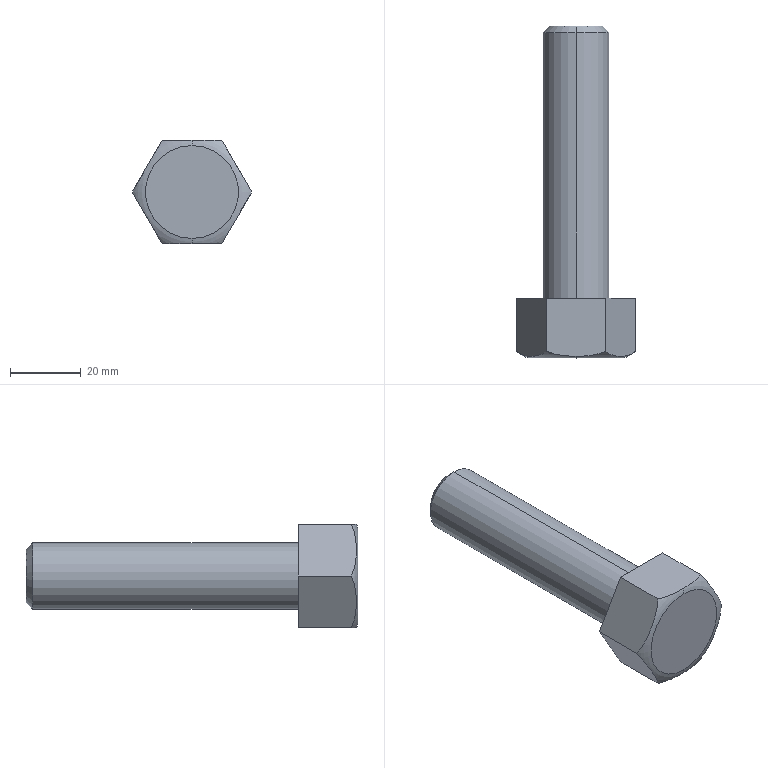Part | SolidWorks | features ICE 1, RevCut 1, Revolution 1, Scale 1 | 1 solid | 15 faces | box 33.75 x 93.75 x 29.228 mm | volume 33536 mm3 | plane 9 | torus 2 | cone 2 | cylinder 2 | commonest cylinder face diameters 18.75 x2
STEP:
#1=CARTESIAN_POINT('',(0.,-17.243,14.614));
#2=VERTEX_POINT('',#1);
#3=CARTESIAN_POINT('',(8.437,-15.803,14.614));
#4=VERTEX_POINT('',#3);
#5=CARTESIAN_POINT('',(0.,-17.243,14.614));
#6=CARTESIAN_POINT('',(0.7213,-17.243,14.614));
#7=CARTESIAN_POINT('',(1.44,-17.222,14.614));
#8=CARTESIAN_POINT('',(2.869,-17.131,14.614));
#9=CARTESIAN_POINT('',(3.581,-17.062,14.614));
#10=CARTESIAN_POINT('',(4.995,-16.856,14.614));
#11=CARTESIAN_POINT('',(5.697,-16.719,14.614));
#12=CARTESIAN_POINT('',(6.739,-16.44,14.614));
#13=CARTESIAN_POINT('',(7.085,-16.334,14.614));
#14=CARTESIAN_POINT('',(7.772,-16.091,14.614));
#15=CARTESIAN_POINT('',(8.109,-15.955,14.614));
#16=CARTESIAN_POINT('',(8.437,-15.803,14.614));
#17=B_SPLINE_CURVE_WITH_KNOTS('',3,(#5,#6,#7,#8,#9,#10,#11,#12,#13,#14,#15,#16),.UNSPECIFIED.,.F.,.F.,(4,2,2,2,2,4),(0.,0.002143,0.004286,0.006428,0.0075,0.008571),.UNSPECIFIED.);
#18=EDGE_CURVE('',#2,#4,#17,.T.);
#19=ORIENTED_EDGE('',*,*,#18,.F.);
#20=CARTESIAN_POINT('',(0.,-17.678,13.125));
#21=VERTEX_POINT('',#20);
#22=CARTESIAN_POINT('',(0.,-10.3,11.78));
#23=DIRECTION('',(1.,0.,0.));
#24=DIRECTION('',(0.,0.,-1.));
#25=AXIS2_PLACEMENT_3D('',#22,#23,#24);
#26=CIRCLE('',#25,7.5);
#27=EDGE_CURVE('',#2,#21,#26,.T.);
#28=ORIENTED_EDGE('',*,*,#27,.T.);
#29=CARTESIAN_POINT('',(0.,-17.678,-13.125));
#30=VERTEX_POINT('',#29);
#31=CARTESIAN_POINT('',(0.,-17.678,0.));
#32=DIRECTION('',(0.,-1.,0.));
#33=DIRECTION('',(0.,0.,-1.));
#34=AXIS2_PLACEMENT_3D('',#31,#32,#33);
#35=CIRCLE('',#34,13.125);
#36=EDGE_CURVE('',#30,#21,#35,.T.);
#37=ORIENTED_EDGE('',*,*,#36,.F.);
#38=CARTESIAN_POINT('',(0.,-17.243,-14.614));
#39=VERTEX_POINT('',#38);
#40=CARTESIAN_POINT('',(0.,-10.3,-11.78));
#41=DIRECTION('',(-1.,0.,0.));
#42=DIRECTION('',(0.,0.,1.));
#43=AXIS2_PLACEMENT_3D('',#40,#41,#42);
#44=CIRCLE('',#43,7.5);
#45=EDGE_CURVE('',#39,#30,#44,.T.);
#46=ORIENTED_EDGE('',*,*,#45,.F.);
#47=CARTESIAN_POINT('',(8.438,-15.803,-14.614));
#48=VERTEX_POINT('',#47);
#49=CARTESIAN_POINT('',(8.438,-15.803,-14.614));
#50=CARTESIAN_POINT('',(7.784,-16.105,-14.614));
#51=CARTESIAN_POINT('',(7.108,-16.339,-14.614));
#52=CARTESIAN_POINT('',(5.723,-16.713,-14.614));
#53=CARTESIAN_POINT('',(5.012,-16.853,-14.614));
#54=CARTESIAN_POINT('',(3.588,-17.061,-14.614));
#55=CARTESIAN_POINT('',(2.874,-17.131,-14.614));
#56=CARTESIAN_POINT('',(1.798,-17.199,-14.614));
#57=CARTESIAN_POINT('',(1.439,-17.216,-14.614));
#58=CARTESIAN_POINT('',(0.9,-17.232,-14.614));
#59=CARTESIAN_POINT('',(0.7202,-17.237,-14.614));
#60=CARTESIAN_POINT('',(0.3603,-17.242,-14.614));
#61=CARTESIAN_POINT('',(0.179,-17.243,-14.614));
#62=CARTESIAN_POINT('',(0.,-17.243,-14.614));
#63=B_SPLINE_CURVE_WITH_KNOTS('',3,(#49,#50,#51,#52,#53,#54,#55,#56,#57,#58,#59,#60,#61,#62),.UNSPECIFIED.,.F.,.F.,(4,2,2,2,2,2,4),(0.05427,0.05639,0.05852,0.06065,0.06171,0.06224,0.06278),.UNSPECIFIED.);
#64=EDGE_CURVE('',#48,#39,#63,.T.);
#65=ORIENTED_EDGE('',*,*,#64,.F.);
#66=CARTESIAN_POINT('',(16.875,-15.803,0.));
#67=VERTEX_POINT('',#66);
#68=CARTESIAN_POINT('',(16.875,-15.803,0.));
#69=CARTESIAN_POINT('',(16.545,-16.109,-0.5716));
#70=CARTESIAN_POINT('',(16.206,-16.342,-1.159));
#71=CARTESIAN_POINT('',(15.514,-16.715,-2.357));
#72=CARTESIAN_POINT('',(15.162,-16.853,-2.967));
#73=CARTESIAN_POINT('',(14.449,-17.061,-4.201));
#74=CARTESIAN_POINT('',(14.09,-17.132,-4.824));
#75=CARTESIAN_POINT('',(13.373,-17.222,-6.065));
#76=CARTESIAN_POINT('',(13.016,-17.243,-6.685));
#77=CARTESIAN_POINT('',(12.3,-17.243,-7.923));
#78=CARTESIAN_POINT('',(11.943,-17.223,-8.542));
#79=CARTESIAN_POINT('',(11.229,-17.133,-9.78));
#80=CARTESIAN_POINT('',(10.872,-17.063,-10.398));
#81=CARTESIAN_POINT('',(10.159,-16.856,-11.633));
#82=CARTESIAN_POINT('',(9.802,-16.717,-12.25));
#83=CARTESIAN_POINT('',(9.107,-16.343,-13.454));
#84=CARTESIAN_POINT('',(8.767,-16.108,-14.043));
#85=CARTESIAN_POINT('',(8.438,-15.803,-14.614));
#86=B_SPLINE_CURVE_WITH_KNOTS('',3,(#68,#69,#70,#71,#72,#73,#74,#75,#76,#77,#78,#79,#80,#81,#82,#83,#84,#85),.UNSPECIFIED.,.F.,.F.,(4,2,2,2,2,2,2,2,4),(0.00000047,0.002148,0.004296,0.006444,0.008592,0.01074,0.01289,0.01504,0.01718),.UNSPECIFIED.);
#87=EDGE_CURVE('',#67,#48,#86,.T.);
#88=ORIENTED_EDGE('',*,*,#87,.F.);
#89=CARTESIAN_POINT('',(8.437,-15.803,14.614));
#90=CARTESIAN_POINT('',(8.768,-16.109,14.043));
#91=CARTESIAN_POINT('',(9.107,-16.342,13.455));
#92=CARTESIAN_POINT('',(9.798,-16.715,12.257));
#93=CARTESIAN_POINT('',(10.15,-16.853,11.648));
#94=CARTESIAN_POINT('',(10.863,-17.061,10.413));
#95=CARTESIAN_POINT('',(11.223,-17.132,9.79));
#96=CARTESIAN_POINT('',(11.939,-17.222,8.549));
#97=CARTESIAN_POINT('',(12.297,-17.243,7.93));
#98=CARTESIAN_POINT('',(13.012,-17.243,6.691));
#99=CARTESIAN_POINT('',(13.369,-17.223,6.072));
#100=CARTESIAN_POINT('',(14.084,-17.133,4.835));
#101=CARTESIAN_POINT('',(14.441,-17.063,4.217));
#102=CARTESIAN_POINT('',(15.154,-16.856,2.982));
#103=CARTESIAN_POINT('',(15.51,-16.717,2.364));
#104=CARTESIAN_POINT('',(16.205,-16.343,1.16));
#105=CARTESIAN_POINT('',(16.545,-16.108,0.5709));
#106=CARTESIAN_POINT('',(16.875,-15.803,0.));
#107=B_SPLINE_CURVE_WITH_KNOTS('',3,(#89,#90,#91,#92,#93,#94,#95,#96,#97,#98,#99,#100,#101,#102,#103,#104,#105,#106),.UNSPECIFIED.,.F.,.F.,(4,2,2,2,2,2,2,2,4),(0.00000047,0.002148,0.004296,0.006444,0.008592,0.01074,0.01289,0.01504,0.01718),.UNSPECIFIED.);
#108=EDGE_CURVE('',#4,#67,#107,.T.);
#109=ORIENTED_EDGE('',*,*,#108,.F.);
#110=EDGE_LOOP('',(#19,#28,#37,#46,#65,#88,#109));
#111=FACE_OUTER_BOUND('',#110,.T.);
#112=CARTESIAN_POINT('',(0.,-10.3,0.));
#113=DIRECTION('',(0.,-1.,0.));
#114=DIRECTION('',(0.,0.,-1.));
#115=AXIS2_PLACEMENT_3D('',#112,#113,#114);
#116=TOROIDAL_SURFACE('',#115,11.78,7.5);
#117=ADVANCED_FACE('',(#111),#116,.T.);
#118=CARTESIAN_POINT('',(0.,76.072,7.5));
#119=VERTEX_POINT('',#118);
#120=CARTESIAN_POINT('',(0.,76.072,-7.5));
#121=VERTEX_POINT('',#120);
#122=CARTESIAN_POINT('',(0.,76.072,0.));
#123=DIRECTION('',(0.,1.,0.));
#124=DIRECTION('',(0.,0.,1.));
#125=AXIS2_PLACEMENT_3D('',#122,#123,#124);
#126=CIRCLE('',#125,7.5);
#127=EDGE_CURVE('',#119,#121,#126,.T.);
#128=ORIENTED_EDGE('',*,*,#127,.F.);
#129=CARTESIAN_POINT('',(0.,74.197,9.375));
#130=VERTEX_POINT('',#129);
#131=CARTESIAN_POINT('',(0.,74.197,9.375));
#132=DIRECTION('',(0.,-0.7071,0.7071));
#133=VECTOR('',#132,1000.);
#134=LINE('',#131,#133);
#135=EDGE_CURVE('',#119,#130,#134,.T.);
#136=ORIENTED_EDGE('',*,*,#135,.T.);
#137=CARTESIAN_POINT('',(0.,74.197,-9.375));
#138=VERTEX_POINT('',#137);
#139=CARTESIAN_POINT('',(0.,74.197,0.));
#140=DIRECTION('',(0.,1.,0.));
#141=DIRECTION('',(0.,0.,1.));
#142=AXIS2_PLACEMENT_3D('',#139,#140,#141);
#143=CIRCLE('',#142,9.375);
#144=EDGE_CURVE('',#130,#138,#143,.T.);
#145=ORIENTED_EDGE('',*,*,#144,.T.);
#146=CARTESIAN_POINT('',(0.,74.197,-9.375));
#147=DIRECTION('',(0.,-0.7071,-0.7071));
#148=VECTOR('',#147,1000.);
#149=LINE('',#146,#148);
#150=EDGE_CURVE('',#121,#138,#149,.T.);
#151=ORIENTED_EDGE('',*,*,#150,.F.);
#152=EDGE_LOOP('',(#128,#136,#145,#151));
#153=FACE_OUTER_BOUND('',#152,.T.);
#154=CARTESIAN_POINT('',(0.,74.197,0.));
#155=DIRECTION('',(0.,-1.,0.));
#156=DIRECTION('',(0.,0.,-1.));
#157=AXIS2_PLACEMENT_3D('',#154,#155,#156);
#158=CONICAL_SURFACE('',#157,9.375,0.7854);
#159=ADVANCED_FACE('',(#153),#158,.T.);
#160=CARTESIAN_POINT('',(0.,-0.803,9.375));
#161=VERTEX_POINT('',#160);
#162=CARTESIAN_POINT('',(0.,-0.803,-9.375));
#163=VERTEX_POINT('',#162);
#164=CARTESIAN_POINT('',(0.,-0.803,0.));
#165=DIRECTION('',(0.,1.,0.));
#166=DIRECTION('',(0.,0.,1.));
#167=AXIS2_PLACEMENT_3D('',#164,#165,#166);
#168=CIRCLE('',#167,9.375);
#169=EDGE_CURVE('',#161,#163,#168,.T.);
#170=ORIENTED_EDGE('',*,*,#169,.T.);
#171=CARTESIAN_POINT('',(0.,76.072,-9.375));
#172=DIRECTION('',(0.,1.,0.));
#173=VECTOR('',#172,1000.);
#174=LINE('',#171,#173);
#175=EDGE_CURVE('',#163,#138,#174,.T.);
#176=ORIENTED_EDGE('',*,*,#175,.T.);
#177=ORIENTED_EDGE('',*,*,#144,.F.);
#178=CARTESIAN_POINT('',(0.,76.072,9.375));
#179=DIRECTION('',(0.,1.,0.));
#180=VECTOR('',#179,1000.);
#181=LINE('',#178,#180);
#182=EDGE_CURVE('',#161,#130,#181,.T.);
#183=ORIENTED_EDGE('',*,*,#182,.F.);
#184=EDGE_LOOP('',(#170,#176,#177,#183));
#185=FACE_OUTER_BOUND('',#184,.T.);
#186=CARTESIAN_POINT('',(0.,76.072,0.));
#187=DIRECTION('',(0.,1.,0.));
#188=DIRECTION('',(0.,0.,1.));
#189=AXIS2_PLACEMENT_3D('',#186,#187,#188);
#190=CYLINDRICAL_SURFACE('',#189,9.375);
#191=ADVANCED_FACE('',(#185),#190,.T.);
#192=CARTESIAN_POINT('',(16.875,-0.803,0.));
#193=VERTEX_POINT('',#192);
#194=CARTESIAN_POINT('',(16.875,1.072,0.));
#195=DIRECTION('',(0.,-1.,0.));
#196=VECTOR('',#195,1000.);
#197=LINE('',#194,#196);
#198=EDGE_CURVE('',#193,#67,#197,.T.);
#199=ORIENTED_EDGE('',*,*,#198,.T.);
#200=ORIENTED_EDGE('',*,*,#87,.T.);
#201=CARTESIAN_POINT('',(8.438,-0.803,-14.614));
#202=VERTEX_POINT('',#201);
#203=CARTESIAN_POINT('',(8.438,1.072,-14.614));
#204=DIRECTION('',(0.,-1.,0.));
#205=VECTOR('',#204,1000.);
#206=LINE('',#203,#205);
#207=EDGE_CURVE('',#202,#48,#206,.T.);
#208=ORIENTED_EDGE('',*,*,#207,.F.);
#209=CARTESIAN_POINT('',(16.875,-0.803,0.));
#210=DIRECTION('',(0.5,0.,0.866));
#211=VECTOR('',#210,1000.);
#212=LINE('',#209,#211);
#213=EDGE_CURVE('',#202,#193,#212,.T.);
#214=ORIENTED_EDGE('',*,*,#213,.T.);
#215=EDGE_LOOP('',(#199,#200,#208,#214));
#216=FACE_OUTER_BOUND('',#215,.T.);
#217=CARTESIAN_POINT('',(8.438,1.072,-14.614));
#218=DIRECTION('',(0.866,0.,-0.5));
#219=DIRECTION('',(-0.5,0.,-0.866));
#220=AXIS2_PLACEMENT_3D('',#217,#218,#219);
#221=PLANE('',#220);
#222=ADVANCED_FACE('',(#216),#221,.T.);
#223=ORIENTED_EDGE('',*,*,#207,.T.);
#224=ORIENTED_EDGE('',*,*,#64,.T.);
#225=CARTESIAN_POINT('',(-8.437,-15.803,-14.614));
#226=VERTEX_POINT('',#225);
#227=CARTESIAN_POINT('',(0.,-17.243,-14.614));
#228=CARTESIAN_POINT('',(-0.7213,-17.243,-14.614));
#229=CARTESIAN_POINT('',(-1.44,-17.222,-14.614));
#230=CARTESIAN_POINT('',(-2.869,-17.131,-14.614));
#231=CARTESIAN_POINT('',(-3.581,-17.062,-14.614));
#232=CARTESIAN_POINT('',(-4.995,-16.856,-14.614));
#233=CARTESIAN_POINT('',(-5.697,-16.719,-14.614));
#234=CARTESIAN_POINT('',(-6.739,-16.44,-14.614));
#235=CARTESIAN_POINT('',(-7.085,-16.334,-14.614));
#236=CARTESIAN_POINT('',(-7.772,-16.091,-14.614));
#237=CARTESIAN_POINT('',(-8.109,-15.955,-14.614));
#238=CARTESIAN_POINT('',(-8.437,-15.803,-14.614));
#239=B_SPLINE_CURVE_WITH_KNOTS('',3,(#227,#228,#229,#230,#231,#232,#233,#234,#235,#236,#237,#238),.UNSPECIFIED.,.F.,.F.,(4,2,2,2,2,4),(0.,0.002143,0.004286,0.006428,0.0075,0.008571),.UNSPECIFIED.);
#240=EDGE_CURVE('',#39,#226,#239,.T.);
#241=ORIENTED_EDGE('',*,*,#240,.T.);
#242=CARTESIAN_POINT('',(-8.437,-0.803,-14.614));
#243=VERTEX_POINT('',#242);
#244=CARTESIAN_POINT('',(-8.437,1.072,-14.614));
#245=DIRECTION('',(0.,-1.,0.));
#246=VECTOR('',#245,1000.);
#247=LINE('',#244,#246);
#248=EDGE_CURVE('',#243,#226,#247,.T.);
#249=ORIENTED_EDGE('',*,*,#248,.F.);
#250=CARTESIAN_POINT('',(16.875,-0.803,-14.614));
#251=DIRECTION('',(1.,0.,0.));
#252=VECTOR('',#251,1000.);
#253=LINE('',#250,#252);
#254=EDGE_CURVE('',#243,#202,#253,.T.);
#255=ORIENTED_EDGE('',*,*,#254,.T.);
#256=EDGE_LOOP('',(#223,#224,#241,#249,#255));
#257=FACE_OUTER_BOUND('',#256,.T.);
#258=CARTESIAN_POINT('',(-8.437,1.072,-14.614));
#259=DIRECTION('',(0.,0.,-1.));
#260=DIRECTION('',(-1.,0.,0.));
#261=AXIS2_PLACEMENT_3D('',#258,#259,#260);
#262=PLANE('',#261);
#263=ADVANCED_FACE('',(#257),#262,.T.);
#264=ORIENTED_EDGE('',*,*,#248,.T.);
#265=CARTESIAN_POINT('',(-16.875,-15.803,0.));
#266=VERTEX_POINT('',#265);
#267=CARTESIAN_POINT('',(-8.437,-15.803,-14.614));
#268=CARTESIAN_POINT('',(-8.768,-16.109,-14.043));
#269=CARTESIAN_POINT('',(-9.107,-16.342,-13.455));
#270=CARTESIAN_POINT('',(-9.798,-16.715,-12.257));
#271=CARTESIAN_POINT('',(-10.15,-16.853,-11.648));
#272=CARTESIAN_POINT('',(-10.863,-17.061,-10.413));
#273=CARTESIAN_POINT('',(-11.223,-17.132,-9.79));
#274=CARTESIAN_POINT('',(-11.939,-17.222,-8.549));
#275=CARTESIAN_POINT('',(-12.297,-17.243,-7.93));
#276=CARTESIAN_POINT('',(-13.012,-17.243,-6.691));
#277=CARTESIAN_POINT('',(-13.369,-17.223,-6.072));
#278=CARTESIAN_POINT('',(-14.084,-17.133,-4.835));
#279=CARTESIAN_POINT('',(-14.441,-17.063,-4.217));
#280=CARTESIAN_POINT('',(-15.154,-16.856,-2.982));
#281=CARTESIAN_POINT('',(-15.51,-16.717,-2.364));
#282=CARTESIAN_POINT('',(-16.205,-16.343,-1.16));
#283=CARTESIAN_POINT('',(-16.545,-16.108,-0.5709));
#284=CARTESIAN_POINT('',(-16.875,-15.803,0.));
#285=B_SPLINE_CURVE_WITH_KNOTS('',3,(#267,#268,#269,#270,#271,#272,#273,#274,#275,#276,#277,#278,#279,#280,#281,#282,#283,#284),.UNSPECIFIED.,.F.,.F.,(4,2,2,2,2,2,2,2,4),(0.00000047,0.002148,0.004296,0.006444,0.008592,0.01074,0.01289,0.01504,0.01718),.UNSPECIFIED.);
#286=EDGE_CURVE('',#226,#266,#285,.T.);
#287=ORIENTED_EDGE('',*,*,#286,.T.);
#288=CARTESIAN_POINT('',(-16.875,-0.803,0.));
#289=VERTEX_POINT('',#288);
#290=CARTESIAN_POINT('',(-16.875,1.072,0.));
#291=DIRECTION('',(0.,-1.,0.));
#292=VECTOR('',#291,1000.);
#293=LINE('',#290,#292);
#294=EDGE_CURVE('',#289,#266,#293,.T.);
#295=ORIENTED_EDGE('',*,*,#294,.F.);
#296=CARTESIAN_POINT('',(-8.437,-0.803,-14.614));
#297=DIRECTION('',(0.5,0.,-0.866));
#298=VECTOR('',#297,1000.);
#299=LINE('',#296,#298);
#300=EDGE_CURVE('',#289,#243,#299,.T.);
#301=ORIENTED_EDGE('',*,*,#300,.T.);
#302=EDGE_LOOP('',(#264,#287,#295,#301));
#303=FACE_OUTER_BOUND('',#302,.T.);
#304=CARTESIAN_POINT('',(-16.875,1.072,0.));
#305=DIRECTION('',(-0.866,0.,-0.5));
#306=DIRECTION('',(-0.5,0.,0.866));
#307=AXIS2_PLACEMENT_3D('',#304,#305,#306);
#308=PLANE('',#307);
#309=ADVANCED_FACE('',(#303),#308,.T.);
#310=ORIENTED_EDGE('',*,*,#294,.T.);
#311=CARTESIAN_POINT('',(-8.438,-15.803,14.614));
#312=VERTEX_POINT('',#311);
#313=CARTESIAN_POINT('',(-16.875,-15.803,0.));
#314=CARTESIAN_POINT('',(-16.545,-16.109,0.5716));
#315=CARTESIAN_POINT('',(-16.206,-16.342,1.159));
#316=CARTESIAN_POINT('',(-15.514,-16.715,2.357));
#317=CARTESIAN_POINT('',(-15.162,-16.853,2.967));
#318=CARTESIAN_POINT('',(-14.449,-17.061,4.201));
#319=CARTESIAN_POINT('',(-14.09,-17.132,4.824));
#320=CARTESIAN_POINT('',(-13.373,-17.222,6.065));
#321=CARTESIAN_POINT('',(-13.016,-17.243,6.685));
#322=CARTESIAN_POINT('',(-12.3,-17.243,7.923));
#323=CARTESIAN_POINT('',(-11.943,-17.223,8.542));
#324=CARTESIAN_POINT('',(-11.229,-17.133,9.78));
#325=CARTESIAN_POINT('',(-10.872,-17.063,10.398));
#326=CARTESIAN_POINT('',(-10.159,-16.856,11.633));
#327=CARTESIAN_POINT('',(-9.802,-16.717,12.25));
#328=CARTESIAN_POINT('',(-9.107,-16.343,13.454));
#329=CARTESIAN_POINT('',(-8.767,-16.108,14.043));
#330=CARTESIAN_POINT('',(-8.438,-15.803,14.614));
#331=B_SPLINE_CURVE_WITH_KNOTS('',3,(#313,#314,#315,#316,#317,#318,#319,#320,#321,#322,#323,#324,#325,#326,#327,#328,#329,#330),.UNSPECIFIED.,.F.,.F.,(4,2,2,2,2,2,2,2,4),(0.00000047,0.002148,0.004296,0.006444,0.008592,0.01074,0.01289,0.01504,0.01718),.UNSPECIFIED.);
#332=EDGE_CURVE('',#266,#312,#331,.T.);
#333=ORIENTED_EDGE('',*,*,#332,.T.);
#334=CARTESIAN_POINT('',(-8.438,-0.803,14.614));
#335=VERTEX_POINT('',#334);
#336=CARTESIAN_POINT('',(-8.438,1.072,14.614));
#337=DIRECTION('',(0.,-1.,0.));
#338=VECTOR('',#337,1000.);
#339=LINE('',#336,#338);
#340=EDGE_CURVE('',#335,#312,#339,.T.);
#341=ORIENTED_EDGE('',*,*,#340,.F.);
#342=CARTESIAN_POINT('',(-8.438,-0.803,14.614));
#343=DIRECTION('',(-0.5,0.,-0.866));
#344=VECTOR('',#343,1000.);
#345=LINE('',#342,#344);
#346=EDGE_CURVE('',#335,#289,#345,.T.);
#347=ORIENTED_EDGE('',*,*,#346,.T.);
#348=EDGE_LOOP('',(#310,#333,#341,#347));
#349=FACE_OUTER_BOUND('',#348,.T.);
#350=CARTESIAN_POINT('',(-8.438,1.072,14.614));
#351=DIRECTION('',(-0.866,0.,0.5));
#352=DIRECTION('',(0.5,0.,0.866));
#353=AXIS2_PLACEMENT_3D('',#350,#351,#352);
#354=PLANE('',#353);
#355=ADVANCED_FACE('',(#349),#354,.T.);
#356=ORIENTED_EDGE('',*,*,#340,.T.);
#357=CARTESIAN_POINT('',(-8.438,-15.803,14.614));
#358=CARTESIAN_POINT('',(-7.784,-16.105,14.614));
#359=CARTESIAN_POINT('',(-7.108,-16.339,14.614));
#360=CARTESIAN_POINT('',(-5.723,-16.713,14.614));
#361=CARTESIAN_POINT('',(-5.012,-16.853,14.614));
#362=CARTESIAN_POINT('',(-3.588,-17.061,14.614));
#363=CARTESIAN_POINT('',(-2.874,-17.131,14.614));
#364=CARTESIAN_POINT('',(-1.798,-17.199,14.614));
#365=CARTESIAN_POINT('',(-1.439,-17.216,14.614));
#366=CARTESIAN_POINT('',(-0.9,-17.232,14.614));
#367=CARTESIAN_POINT('',(-0.7202,-17.237,14.614));
#368=CARTESIAN_POINT('',(-0.3603,-17.242,14.614));
#369=CARTESIAN_POINT('',(-0.179,-17.243,14.614));
#370=CARTESIAN_POINT('',(0.,-17.243,14.614));
#371=B_SPLINE_CURVE_WITH_KNOTS('',3,(#357,#358,#359,#360,#361,#362,#363,#364,#365,#366,#367,#368,#369,#370),.UNSPECIFIED.,.F.,.F.,(4,2,2,2,2,2,4),(0.05427,0.05639,0.05852,0.06065,0.06171,0.06224,0.06278),.UNSPECIFIED.);
#372=EDGE_CURVE('',#312,#2,#371,.T.);
#373=ORIENTED_EDGE('',*,*,#372,.T.);
#374=ORIENTED_EDGE('',*,*,#18,.T.);
#375=CARTESIAN_POINT('',(8.437,-0.803,14.614));
#376=VERTEX_POINT('',#375);
#377=CARTESIAN_POINT('',(8.437,1.072,14.614));
#378=DIRECTION('',(0.,-1.,0.));
#379=VECTOR('',#378,1000.);
#380=LINE('',#377,#379);
#381=EDGE_CURVE('',#376,#4,#380,.T.);
#382=ORIENTED_EDGE('',*,*,#381,.F.);
#383=CARTESIAN_POINT('',(16.875,-0.803,14.614));
#384=DIRECTION('',(-1.,0.,0.));
#385=VECTOR('',#384,1000.);
#386=LINE('',#383,#385);
#387=EDGE_CURVE('',#376,#335,#386,.T.);
#388=ORIENTED_EDGE('',*,*,#387,.T.);
#389=EDGE_LOOP('',(#356,#373,#374,#382,#388));
#390=FACE_OUTER_BOUND('',#389,.T.);
#391=CARTESIAN_POINT('',(8.437,1.072,14.614));
#392=DIRECTION('',(0.,0.,1.));
#393=DIRECTION('',(1.,0.,0.));
#394=AXIS2_PLACEMENT_3D('',#391,#392,#393);
#395=PLANE('',#394);
#396=ADVANCED_FACE('',(#390),#395,.T.);
#397=ORIENTED_EDGE('',*,*,#381,.T.);
#398=ORIENTED_EDGE('',*,*,#108,.T.);
#399=ORIENTED_EDGE('',*,*,#198,.F.);
#400=CARTESIAN_POINT('',(16.875,-0.803,0.));
#401=DIRECTION('',(-0.5,0.,0.866));
#402=VECTOR('',#401,1000.);
#403=LINE('',#400,#402);
#404=EDGE_CURVE('',#193,#376,#403,.T.);
#405=ORIENTED_EDGE('',*,*,#404,.T.);
#406=EDGE_LOOP('',(#397,#398,#399,#405));
#407=FACE_OUTER_BOUND('',#406,.T.);
#408=CARTESIAN_POINT('',(16.875,1.072,0.));
#409=DIRECTION('',(0.866,0.,0.5));
#410=DIRECTION('',(0.5,0.,-0.866));
#411=AXIS2_PLACEMENT_3D('',#408,#409,#410);
#412=PLANE('',#411);
#413=ADVANCED_FACE('',(#407),#412,.T.);
#414=ORIENTED_EDGE('',*,*,#169,.F.);
#415=CARTESIAN_POINT('',(0.,-0.803,0.));
#416=DIRECTION('',(0.,1.,0.));
#417=DIRECTION('',(0.,0.,1.));
#418=AXIS2_PLACEMENT_3D('',#415,#416,#417);
#419=CIRCLE('',#418,9.375);
#420=EDGE_CURVE('',#163,#161,#419,.T.);
#421=ORIENTED_EDGE('',*,*,#420,.F.);
#422=EDGE_LOOP('',(#414,#421));
#423=FACE_BOUND('',#422,.T.);
#424=ORIENTED_EDGE('',*,*,#213,.F.);
#425=ORIENTED_EDGE('',*,*,#254,.F.);
#426=ORIENTED_EDGE('',*,*,#300,.F.);
#427=ORIENTED_EDGE('',*,*,#346,.F.);
#428=ORIENTED_EDGE('',*,*,#387,.F.);
#429=ORIENTED_EDGE('',*,*,#404,.F.);
#430=EDGE_LOOP('',(#424,#425,#426,#427,#428,#429));
#431=FACE_OUTER_BOUND('',#430,.T.);
#432=CARTESIAN_POINT('',(16.875,-0.803,0.));
#433=DIRECTION('',(0.,-1.,0.));
#434=DIRECTION('',(0.,0.,-1.));
#435=AXIS2_PLACEMENT_3D('',#432,#433,#434);
#436=PLANE('',#435);
#437=ADVANCED_FACE('',(#423,#431),#436,.F.);
#438=ORIENTED_EDGE('',*,*,#175,.F.);
#439=ORIENTED_EDGE('',*,*,#420,.T.);
#440=ORIENTED_EDGE('',*,*,#182,.T.);
#441=CARTESIAN_POINT('',(0.,74.197,0.));
#442=DIRECTION('',(0.,1.,0.));
#443=DIRECTION('',(0.,0.,1.));
#444=AXIS2_PLACEMENT_3D('',#441,#442,#443);
#445=CIRCLE('',#444,9.375);
#446=EDGE_CURVE('',#138,#130,#445,.T.);
#447=ORIENTED_EDGE('',*,*,#446,.F.);
#448=EDGE_LOOP('',(#438,#439,#440,#447));
#449=FACE_OUTER_BOUND('',#448,.T.);
#450=CARTESIAN_POINT('',(0.,76.072,0.));
#451=DIRECTION('',(0.,1.,0.));
#452=DIRECTION('',(0.,0.,1.));
#453=AXIS2_PLACEMENT_3D('',#450,#451,#452);
#454=CYLINDRICAL_SURFACE('',#453,9.375);
#455=ADVANCED_FACE('',(#449),#454,.T.);
#456=ORIENTED_EDGE('',*,*,#135,.F.);
#457=CARTESIAN_POINT('',(0.,76.072,0.));
#458=DIRECTION('',(0.,1.,0.));
#459=DIRECTION('',(0.,0.,1.));
#460=AXIS2_PLACEMENT_3D('',#457,#458,#459);
#461=CIRCLE('',#460,7.5);
#462=EDGE_CURVE('',#121,#119,#461,.T.);
#463=ORIENTED_EDGE('',*,*,#462,.F.);
#464=ORIENTED_EDGE('',*,*,#150,.T.);
#465=ORIENTED_EDGE('',*,*,#446,.T.);
#466=EDGE_LOOP('',(#456,#463,#464,#465));
#467=FACE_OUTER_BOUND('',#466,.T.);
#468=CARTESIAN_POINT('',(0.,74.197,0.));
#469=DIRECTION('',(0.,-1.,0.));
#470=DIRECTION('',(0.,0.,-1.));
#471=AXIS2_PLACEMENT_3D('',#468,#469,#470);
#472=CONICAL_SURFACE('',#471,9.375,0.7854);
#473=ADVANCED_FACE('',(#467),#472,.T.);
#474=ORIENTED_EDGE('',*,*,#462,.T.);
#475=ORIENTED_EDGE('',*,*,#127,.T.);
#476=EDGE_LOOP('',(#474,#475));
#477=FACE_OUTER_BOUND('',#476,.T.);
#478=CARTESIAN_POINT('',(7.5,76.072,0.));
#479=DIRECTION('',(0.,-1.,0.));
#480=DIRECTION('',(0.,0.,-1.));
#481=AXIS2_PLACEMENT_3D('',#478,#479,#480);
#482=PLANE('',#481);
#483=ADVANCED_FACE('',(#477),#482,.F.);
#484=ORIENTED_EDGE('',*,*,#27,.F.);
#485=ORIENTED_EDGE('',*,*,#372,.F.);
#486=ORIENTED_EDGE('',*,*,#332,.F.);
#487=ORIENTED_EDGE('',*,*,#286,.F.);
#488=ORIENTED_EDGE('',*,*,#240,.F.);
#489=ORIENTED_EDGE('',*,*,#45,.T.);
#490=CARTESIAN_POINT('',(0.,-17.678,0.));
#491=DIRECTION('',(0.,-1.,0.));
#492=DIRECTION('',(0.,0.,-1.));
#493=AXIS2_PLACEMENT_3D('',#490,#491,#492);
#494=CIRCLE('',#493,13.125);
#495=EDGE_CURVE('',#21,#30,#494,.T.);
#496=ORIENTED_EDGE('',*,*,#495,.F.);
#497=EDGE_LOOP('',(#484,#485,#486,#487,#488,#489,#496));
#498=FACE_OUTER_BOUND('',#497,.T.);
#499=CARTESIAN_POINT('',(0.,-10.3,0.));
#500=DIRECTION('',(0.,-1.,0.));
#501=DIRECTION('',(0.,0.,-1.));
#502=AXIS2_PLACEMENT_3D('',#499,#500,#501);
#503=TOROIDAL_SURFACE('',#502,11.78,7.5);
#504=ADVANCED_FACE('',(#498),#503,.T.);
#505=ORIENTED_EDGE('',*,*,#36,.T.);
#506=ORIENTED_EDGE('',*,*,#495,.T.);
#507=EDGE_LOOP('',(#505,#506));
#508=FACE_OUTER_BOUND('',#507,.T.);
#509=CARTESIAN_POINT('',(0.,-17.678,0.));
#510=DIRECTION('',(0.,1.,0.));
#511=DIRECTION('',(0.,0.,1.));
#512=AXIS2_PLACEMENT_3D('',#509,#510,#511);
#513=PLANE('',#512);
#514=ADVANCED_FACE('',(#508),#513,.F.);
#515=CLOSED_SHELL('',(#117,#159,#191,#222,#263,#309,#355,#396,#413,#437,#455,#473,#483,#504,#514));
#516=MANIFOLD_SOLID_BREP('',#515);
#517=CARTESIAN_POINT('',(0.,0.,0.));
#518=DIRECTION('',(0.,0.,1.));
#519=DIRECTION('',(1.,0.,0.));
#520=AXIS2_PLACEMENT_3D('',#517,#518,#519);
#521=(LENGTH_UNIT()NAMED_UNIT(*)SI_UNIT(.MILLI.,.METRE.));
#522=UNCERTAINTY_MEASURE_WITH_UNIT(LENGTH_MEASURE(0.00001),#521,'','');
#523=(NAMED_UNIT(*)PLANE_ANGLE_UNIT()SI_UNIT($,.RADIAN.));
#524=(NAMED_UNIT(*)SI_UNIT($,.STERADIAN.)SOLID_ANGLE_UNIT());
#525=(GEOMETRIC_REPRESENTATION_CONTEXT(3)GLOBAL_UNCERTAINTY_ASSIGNED_CONTEXT((#522))GLOBAL_UNIT_ASSIGNED_CONTEXT((#521,#523,#524))REPRESENTATION_CONTEXT('',''));
#526=ADVANCED_BREP_SHAPE_REPRESENTATION('',(#516,#520),#525);